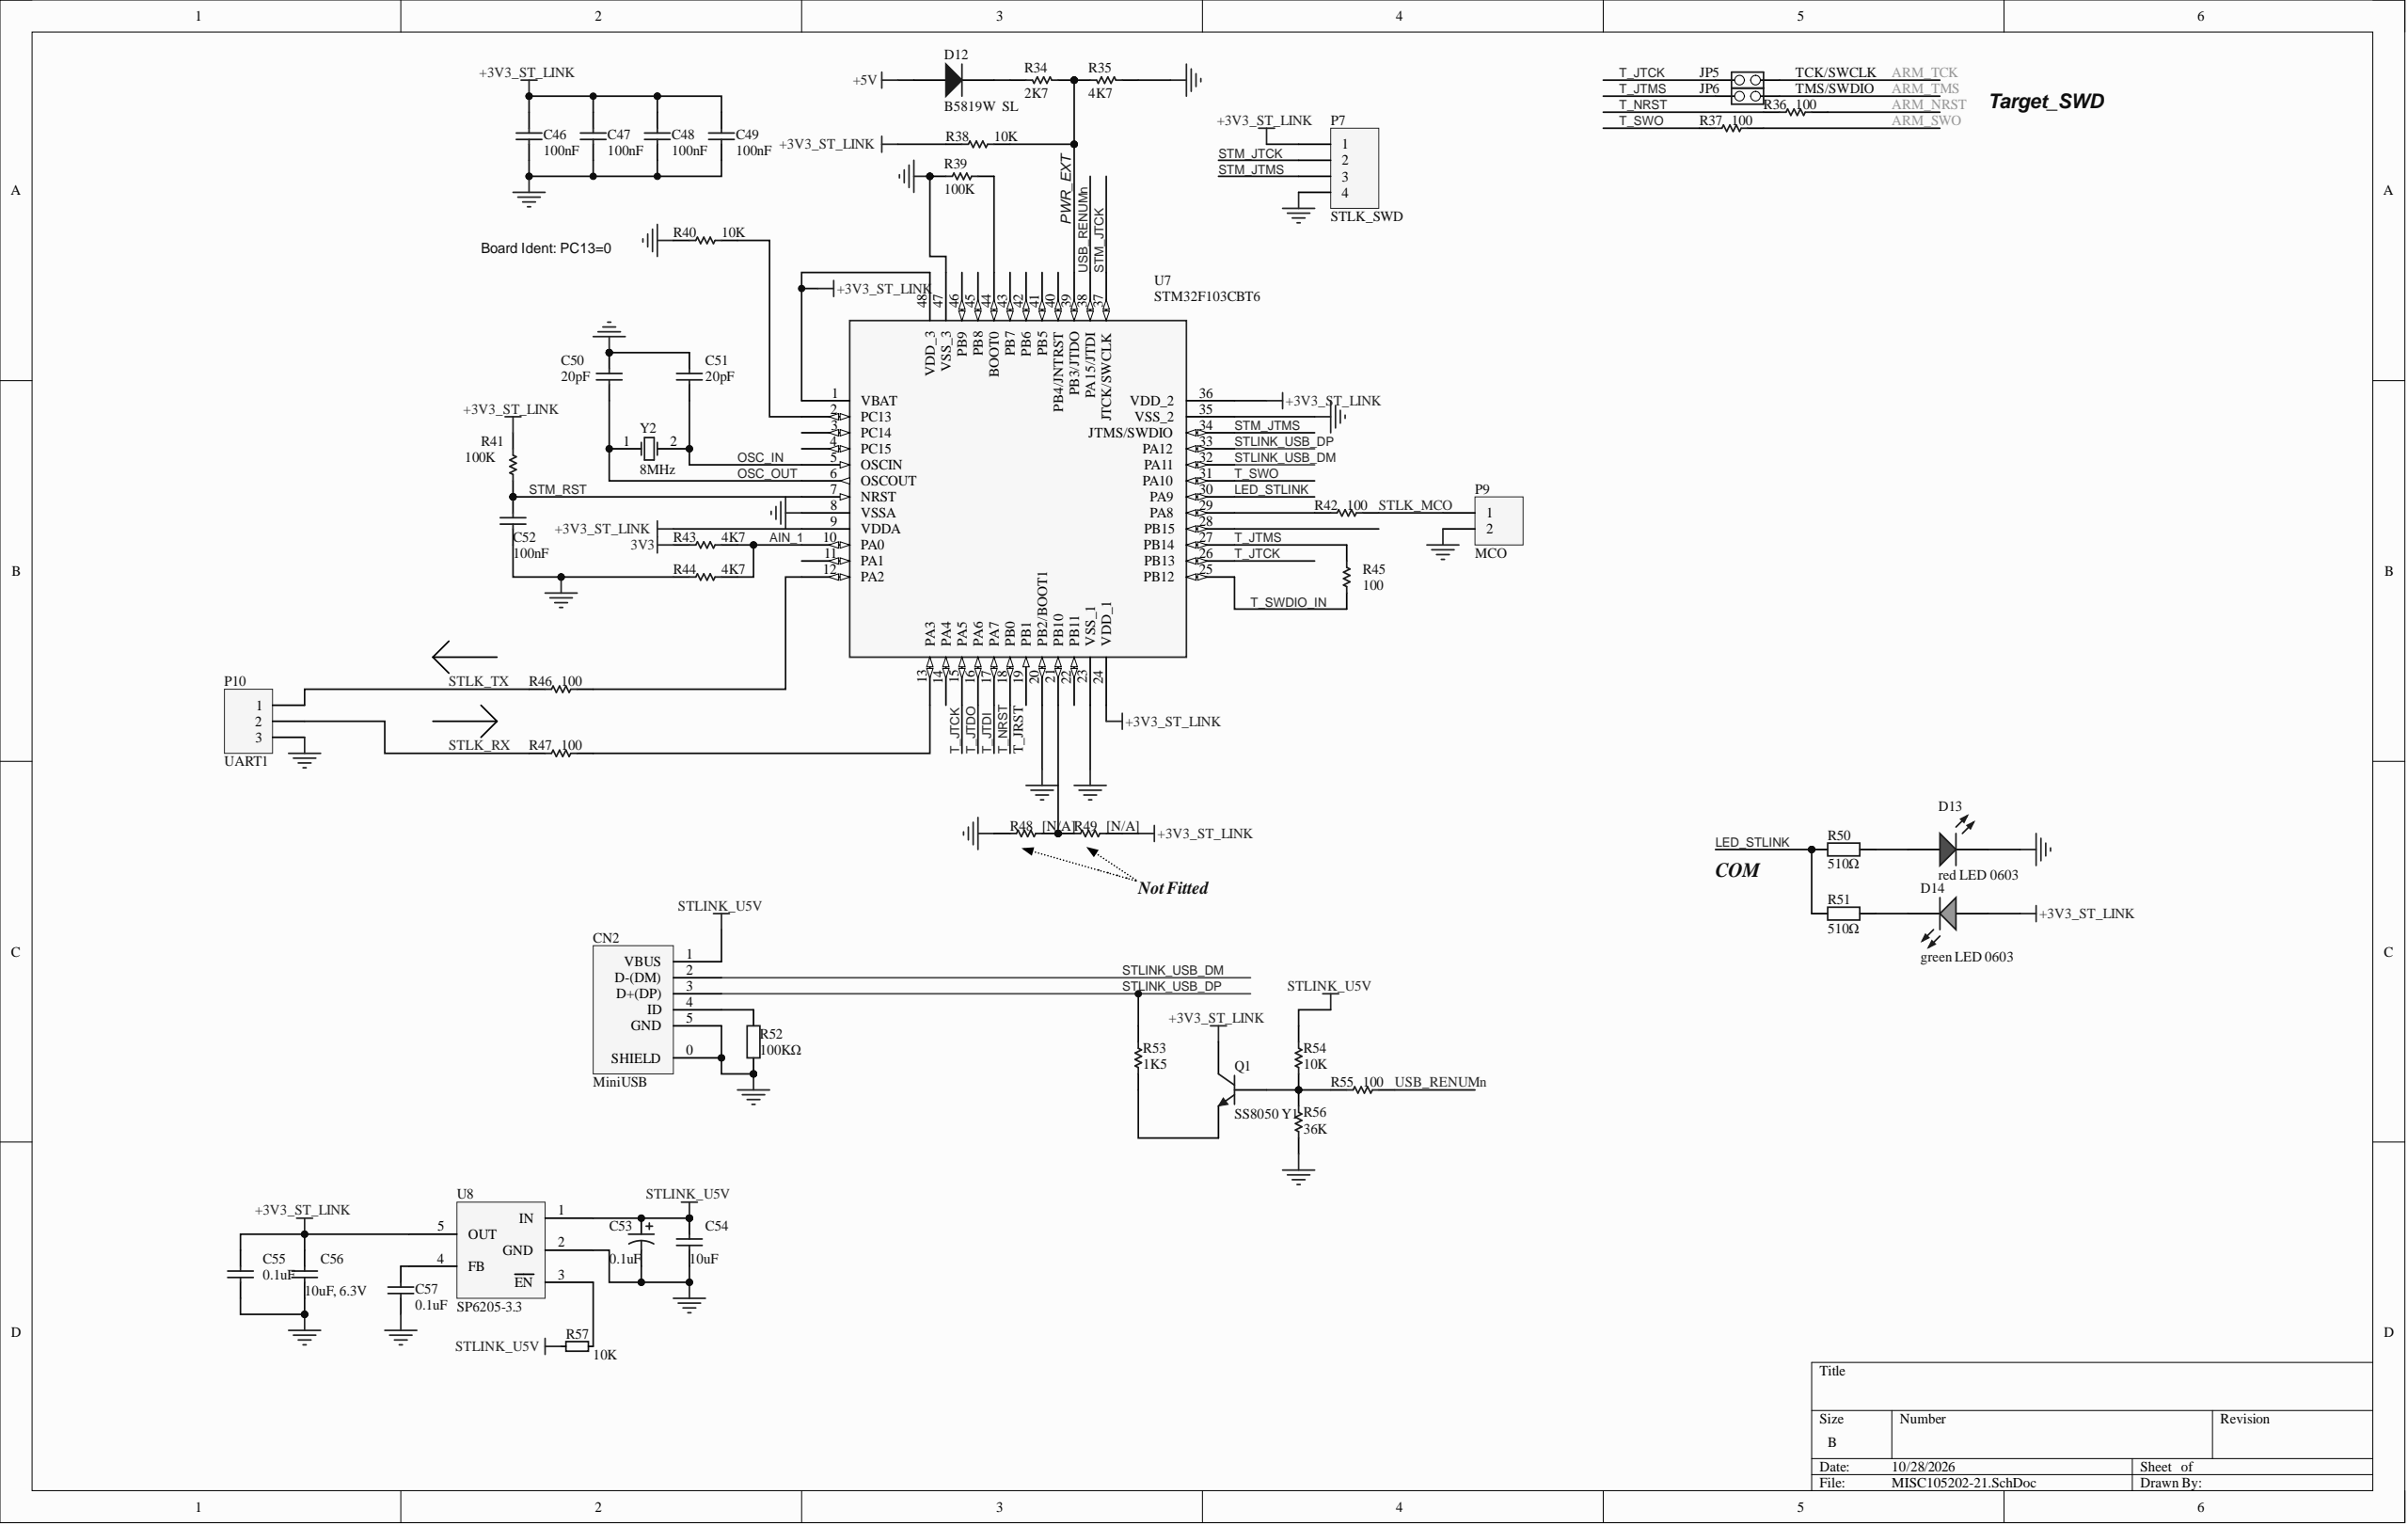Circuit board | Altium Designer | 181 parts | 141 nets | one sheet of the schematic
Parts on this sheet (reference | value | footprint):
C46 | 100nF | 0603_C
C47 | 100nF | 0603_C
C48 | 100nF | 0603_C
C49 | 100nF | 0603_C
C50 | 20pF | 0603_C
C51 | 20pF | 0603_C
C52 | 100nF | 0603_C
C53 | 0.1uF | 0402_C
C54 | 10uF | 0402_C
C55 | 0.1uF,25V | 0603_C
C56 | 10uF, 6.3V | 0402_C
C57 | 0.1uF | 0402_C
CN2 | MiniUSB | Mini-USB-AB
D12 | B5819W  SL | SOD-123
D13 | red LED 0603 | 0603_LED_S1
D14 | green LED 0603 | 0603_LED_S1
JP5 | HDR1X2
JP6 | HDR1X2
P7 | STLK_SWD | 127*4
P9 | MCO | HDR1X2
P10 | UART1 | HDR1X3
Q1 | SS8050 Y1 | SOT-23(SOT-23-3)
R34 | 2K7 | 0603_R
R35 | 4K7 | 0603_R
R36 | 100 | 0603_R
R37 | 100 | 0603_R
R38 | 10K | 0603_R
R39 | 100K | 0603_R
R40 | 10K | 0603_R
R41 | 100K | 0603_R
R42 | 100 | 0603_R
R43 | 4K7 | 0603_R
R44 | 4K7 | 0603_R
R45 | 100 | 0603_R
R46 | 100 | 0603_R
R47 | 100 | 0603_R
R48 | [N/A] | 0603_R
R49 | [N/A] | 0603_R
R50 | 510Ω | 0603_R
R51 | 510Ω | 0603_R
R52 | 100KΩ | 0603_R
R53 | 1K5 | 0603_R
R54 | 10K | 0603_R
R55 | 100 | 0603_R
R56 | 36K | 0603_R
R57 | 10K | 0402_R
U7 | STM32F103CBT6 | LQFP-48_7x7x05P
U8 | SP6205-3.3 | SOT23-5
Y2 | 8MHz | SMD-5032_2P
Nets of these parts (net: part-pin ...):
USB_RENUMn: R55-2 U7-38
T_SWO: R37-1 U7-31
T_SWDIO_IN: R45-1 U7-25
T_NRST: R36-1 U7-18
T_JTMS: JP6-1 R45-2 U7-27
T_JTCK: JP5-1 U7-15 U7-26
STM_RST: C52-2 R41-1 U7-7
STM_JTMS: P7-3 U7-34
STM_JTCK: P7-2 U7-37
STLK_MCO: P9-1 R42-2
STLINK_USB_DP: CN2-3 R53-1 U7-33
STLINK_USB_DM: CN2-2 U7-32
STLINK_U5V: C53-1 C54-2 CN2-1 R54-2 R57-2 U8-1
PA10_U1R: P10-1 R46-1
PA9_U1T: P10-2 R47-1
OSC_OUT: C50-1 Y2-1 U7-6
OSC_IN: C51-1 Y2-2 U7-5
NetR57_1: R57-1 U8-3
NetR48_1: R48-1 R49-2 U7-21
NetR47_2: R47-2 U7-13
NetR46_2: R46-2 U7-12
NetR42_1: R42-1 U7-29
NetR40_2: R40-2 U7-2
NetR39_2: R39-2 U7-44
NetR34_2: R34-2 R35-1 R38-2 U7-39
NetQ1_2: Q1-2 R53-2
NetQ1_1: Q1-1 R54-1 R55-1 R56-2
NetD14_K: D14-K R51-2
NetD13_A: D13-A R50-2
NetD12_2: D12-2 R34-1
NetCN2_4: CN2-4 R52-2
NetC57_2: C57-2 U8-4
LED_STLINK: R50-1 R51-1 U7-30
GND: C46-1 C47-1 C48-1 C49-1 C50-2 C51-2 C52-1 C53-2 C54-1 C55-1 C56-1 C57-1 CN2-0 CN2-5 D13-K P7-4 P9-2 P10-3 R35-2 R39-1 R40-1 R44-1 R48-2 R52-1 R56-1 U8-2 U7-8 U7-20 U7-23 U7-35 U7-47
ARM_TMS: JP6-2
ARM_TCK: JP5-2
ARM_NRST: R36-2
AIN_1: R43-2 R44-2 U7-10
+5V: D12-1
+3V3_ST_LINK: C46-2 C47-2 C48-2 C49-2 C55-2 C56-2 D14-A P7-1 Q1-3 R38-1 R41-2 R49-1 U8-5 U7-1 U7-9 U7-24 U7-36 U7-48
3V3: R43-1